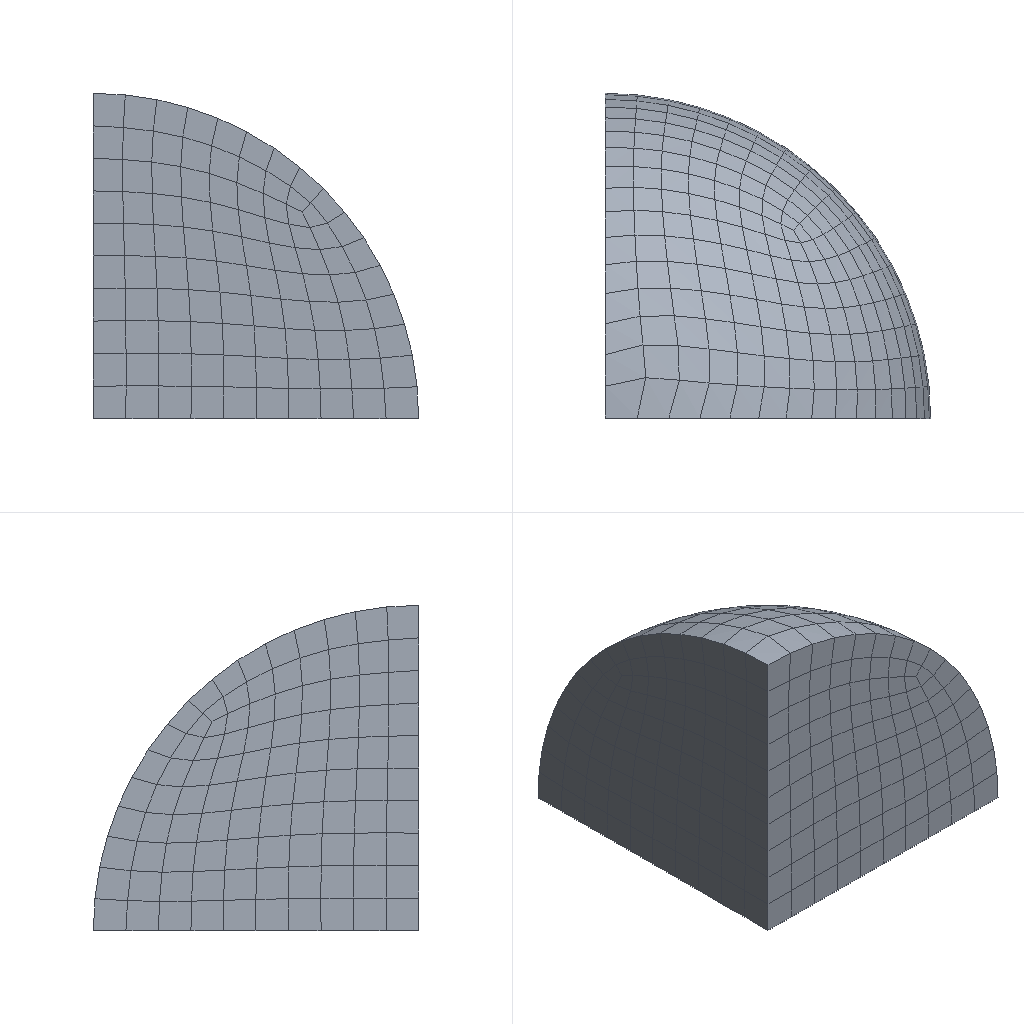Simulation study | abaqus
Set-up summary:
category,name,step,type,value,unit,region
solver,abaqus,,Abaqus/CAE 2024
units,mm-N-s-tonne (MPa),,inferred,E=10000 density=
analysis,load,,soils,time_period=0.001
analysis,consolidation,,soils,time_period=72
mesh,nodes,,,1163
mesh,elements,,,896
element_type,C3D8P,,,896
material,soil,,E,10000
material,soil,,nu,0.3
section,soil,,solid section,,,_PickedSet6
load,Predefined,initial,initial condition ratio
load,Load-1,load,pressure,100,,_PickedSurf10
bc,BC-1,initial,fixed,[dofs=x],,_PickedSet11
bc,BC-2,initial,fixed,[dofs=z],,_PickedSet12
bc,BC-3,initial,fixed,[dofs=y],,_PickedSet13
bc,BC-4,consolidation,fixed,[dofs=8],,_PickedSet14_PP_
Abaqus input file, long lists of numbers shortened:
*Heading
** Job name: deck Model name: Model-1
** Generated by: Abaqus/CAE 2024
*Preprint, echo=NO, model=NO, history=NO, contact=NO
**
** PARTS
**
*Part, name=Part-1
*Node
      1,   3.536,   3.536,           0.
      2,           0.,           5.,           0.
** (1161 more lines like these left out)
*Element, type=C3D8P
  1,   73,  282,  674,  268,    1,   16,  170,   43
  2,  282,  283,  675,  674,   16,   17,  171,  170
** (894 more lines like these left out)
*Nset, nset=_PickedSet6, internal, generate
    1,  1163,     1
*Elset, elset=_PickedSet6, internal, generate
   1,  896,    1
** Section: soil
*Solid Section, elset=_PickedSet6, material=soil
,
*End Part
**
**
** ASSEMBLY
**
*Assembly, name=Assembly
**
*Instance, name=Part-1-1, part=Part-1
*End Instance
**
*Nset, nset=_PickedSet11, internal, instance=Part-1-1
   2,   3,   6,   7,   9,  11,  15,  23,  24,  25,  26,  27,  28,  29,  51,  52
  53,  54,  55,  56,  57,  74,  75,  76,  77,  78,  79,  80,  81,  82,  97,  98
** (6 more lines like these left out)
*Elset, elset=_PickedSet11, internal, instance=Part-1-1
   8,  16,  24,  32,  40,  48,  56,  64,  72,  80,  88,  96, 104, 112, 120, 128
 129, 130, 131, 132, 133, 134, 135, 136, 193, 194, 195, 196, 197, 198, 199, 200
** (4 more lines like these left out)
*Nset, nset=_PickedSet12, internal, instance=Part-1-1
   1,   2,   5,   6,  13,  14,  15,  16,  17,  18,  19,  20,  21,  22,  44,  45
  46,  47,  48,  49,  50,  73,  75, 127, 128, 129, 130, 131, 132, 133, 141, 142
** (6 more lines like these left out)
*Elset, elset=_PickedSet12, internal, instance=Part-1-1
   1,   2,   3,   4,   5,   6,   7,   8,  65,  66,  67,  68,  69,  70,  71,  72
 264, 272, 280, 288, 296, 304, 312, 320, 328, 336, 344, 352, 360, 368, 376, 384
** (4 more lines like these left out)
*Nset, nset=_PickedSet13, internal, instance=Part-1-1
   9,  10,  11,  12,  13,  14,  15,  83,  84,  85,  86,  87,  88,  89, 104, 105
 106, 107, 108, 109, 110, 118, 119, 120, 121, 122, 123, 124, 125, 126, 134, 135
** (6 more lines like these left out)
*Elset, elset=_PickedSet13, internal, instance=Part-1-1
 136, 144, 152, 160, 168, 176, 184, 192, 200, 208, 216, 224, 232, 240, 248, 256
 257, 258, 259, 260, 261, 262, 263, 264, 321, 322, 323, 324, 325, 326, 327, 328
** (4 more lines like these left out)
*Nset, nset=_PickedSet14, internal, instance=Part-1-1
   1,   2,   3,   4,   9,  10,  13,  16,  17,  18,  19,  20,  21,  22,  23,  24
  25,  26,  27,  28,  29,  30,  31,  32,  33,  34,  35,  36,  37,  38,  39,  40
** (12 more lines like these left out)
*Elset, elset=_PickedSet14, internal, instance=Part-1-1
   1,   2,   3,   4,   5,   6,   7,   8,   9,  10,  11,  12,  13,  14,  15,  16
  17,  18,  19,  20,  21,  22,  23,  24,  25,  26,  27,  28,  29,  30,  31,  32
** (10 more lines like these left out)
*Nset, nset=_PickedSet15, internal, instance=Part-1-1, generate
    1,  1163,     1
*Elset, elset=_PickedSet15, internal, instance=Part-1-1, generate
   1,  896,    1
*Elset, elset=__PickedSurf10_S2, internal, instance=Part-1-1
   1,   2,   3,   4,   5,   6,   7,   8,   9,  10,  11,  12,  13,  14,  15,  16
  17,  18,  19,  20,  21,  22,  23,  24,  25,  26,  27,  28,  29,  30,  31,  32
** (10 more lines like these left out)
*Surface, type=ELEMENT, name=_PickedSurf10, internal
__PickedSurf10_S2, S2
*Nset, nset=_PickedSet14_PP_, internal, instance=Part-1-1
   1,   2,   3,   4,   9,  10,  13,  16,  17,  18,  19,  20,  21,  22,  23,  24
  25,  26,  27,  28,  29,  30,  31,  32,  33,  34,  35,  36,  37,  38,  39,  40
** (12 more lines like these left out)
*End Assembly
**
** MATERIALS
**
*Material, name=soil
*Elastic
10000., 0.3
*Permeability, specific=10.
 3.6e-05,0.
**
** BOUNDARY CONDITIONS
**
** Name: BC-1 Type: Displacement/Rotation
*Boundary
_PickedSet11, 1, 1
** Name: BC-2 Type: Displacement/Rotation
*Boundary
_PickedSet12, 3, 3
** Name: BC-3 Type: Displacement/Rotation
*Boundary
_PickedSet13, 2, 2
**
** PREDEFINED FIELDS
**
** Name: Predefined Field-1   Type: Void ratio
*Initial Conditions, TYPE=RATIO
_PickedSet15, 1.
** ----------------------------------------------------------------
**
** STEP: load
**
*Step, name=load, nlgeom=NO
*Soils, consolidation, end=PERIOD, creep=none
0.001, 0.001, , ,
**
** LOADS
**
** Name: Load-1   Type: Pressure
*Dsload
_PickedSurf10, P, 100.
**
** OUTPUT REQUESTS
**
*Restart, write, frequency=0
**
** FIELD OUTPUT: F-Output-1
**
*Output, field, variable=PRESELECT
**
** HISTORY OUTPUT: H-Output-1
**
*Output, history, variable=PRESELECT
*End Step
** ----------------------------------------------------------------
**
** STEP: consolidation
**
*Step, name=consolidation, nlgeom=NO
*Soils, consolidation, end=PERIOD, utol=100., creep=none
1., 72., 0.00072, 5.,
**
** BOUNDARY CONDITIONS
**
** Name: BC-4 Type: Pore pressure
*Boundary
_PickedSet14_PP_, 8, 8
**
** OUTPUT REQUESTS
**
*Restart, write, frequency=0
**
** FIELD OUTPUT: F-Output-1
**
*Output, field, variable=PRESELECT
**
** HISTORY OUTPUT: H-Output-1
**
*Output, history, variable=PRESELECT
*End Step
Results summary:
result,odb.job_status,,,JOB_STATUS_COMPLETED_SUCCESSFULLY,"consistent, unstated (Abaqus has no unit system)"
result,steps[0].procedure,load,,"*SOILS, CONSOLIDATION","consistent, unstated (Abaqus has no unit system)"
result,steps[0].time_period,load,,0.001,"consistent, unstated (Abaqus has no unit system)"
result,steps[0].n_frames,load,,2,"consistent, unstated (Abaqus has no unit system)"
result,steps[0].last_frame.id,load,,1,"consistent, unstated (Abaqus has no unit system)"
result,steps[0].last_frame.value,load,,0.001,"consistent, unstated (Abaqus has no unit system)"
result,steps[0].last_frame.description,load,,Increment      1: Step Time =   1.0000E-03,"consistent, unstated (Abaqus has no unit system)"
result,steps[0].completed,load,,True,"consistent, unstated (Abaqus has no unit system)"
result,steps[0].max_U_magnitude,load,,1.87567e-17,"consistent, unstated (Abaqus has no unit system)"
result,steps[0].max_S_mises,load,,2.56952e-13,"consistent, unstated (Abaqus has no unit system)"
result,steps[0].RF_sum[1],load,,1960.34,"consistent, unstated (Abaqus has no unit system)"
result,steps[0].RF_sum[2],load,,1960.34,"consistent, unstated (Abaqus has no unit system)"
result,steps[0].RF_sum[3],load,,1960.34,"consistent, unstated (Abaqus has no unit system)"
result,steps[1].procedure,consolidation,,"*SOILS, CONSOLIDATION","consistent, unstated (Abaqus has no unit system)"
result,steps[1].time_period,consolidation,,72,"consistent, unstated (Abaqus has no unit system)"
result,steps[1].n_frames,consolidation,,19,"consistent, unstated (Abaqus has no unit system)"
result,steps[1].last_frame.id,consolidation,,18,"consistent, unstated (Abaqus has no unit system)"
result,steps[1].last_frame.value,consolidation,,72,"consistent, unstated (Abaqus has no unit system)"
result,steps[1].last_frame.description,consolidation,,Increment     18: Step Time =    72.00,"consistent, unstated (Abaqus has no unit system)"
result,steps[1].completed,consolidation,,True,"consistent, unstated (Abaqus has no unit system)"
result,steps[1].max_U_magnitude,consolidation,,0.01437,"consistent, unstated (Abaqus has no unit system)"
result,steps[1].max_S_mises,consolidation,,15.949,"consistent, unstated (Abaqus has no unit system)"
result,steps[1].RF_sum[1],consolidation,,1960.34,"consistent, unstated (Abaqus has no unit system)"
result,steps[1].RF_sum[2],consolidation,,1960.34,"consistent, unstated (Abaqus has no unit system)"
result,steps[1].RF_sum[3],consolidation,,1960.34,"consistent, unstated (Abaqus has no unit system)"